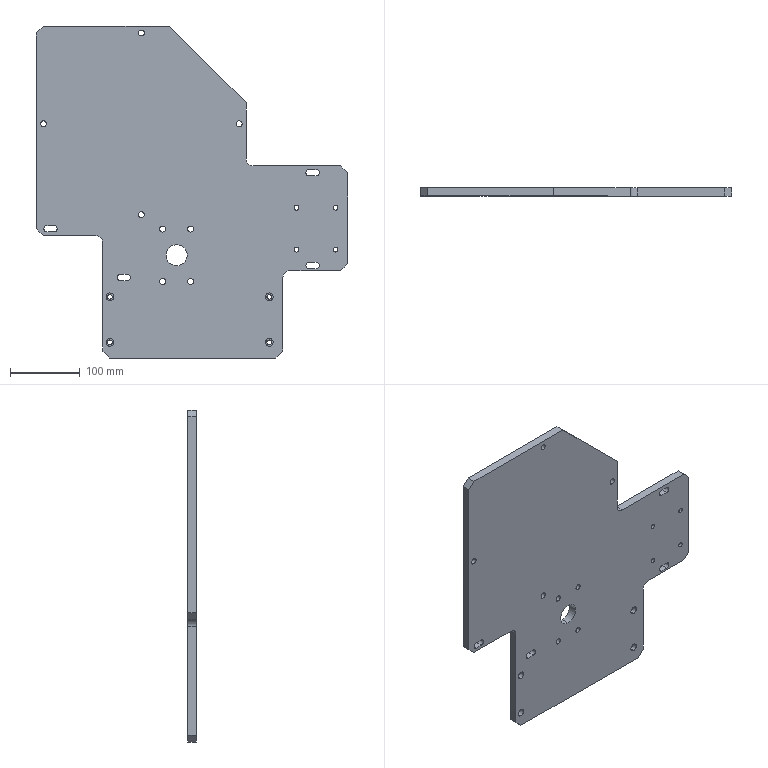Part | STEP file | PN_0001 | 1 solid | 116 faces | box 445 x 12 x 475 mm | volume 1746593 mm3 | cylinder 69 | plane 31 | cone 16 | commonest cylinder face diameters 8.5 x16 5 x12 6.6 x8 6.8 x8 9 x8 11 x8